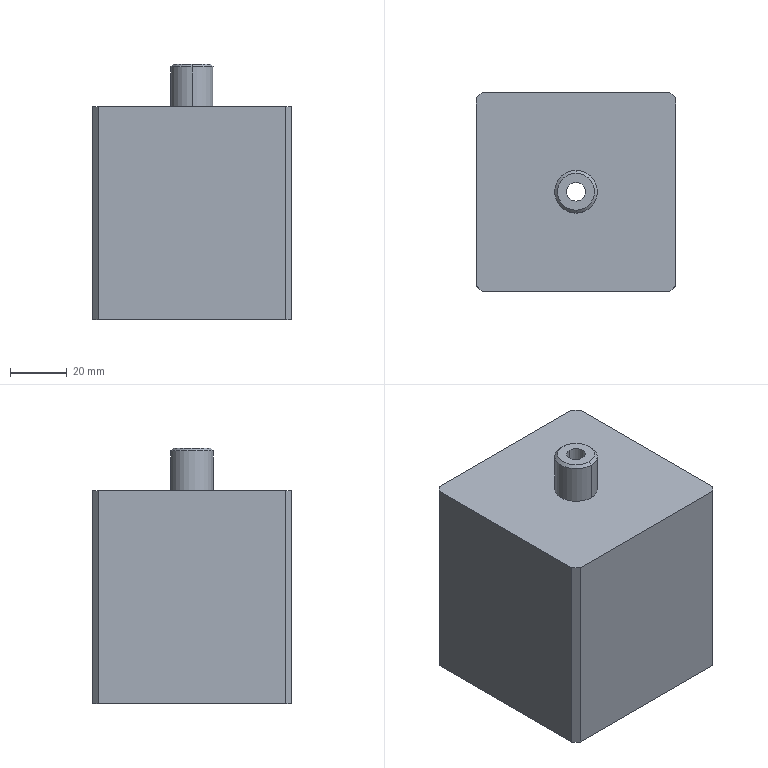NC program | NX | posted with a generic post | part box 70 x 70 x 90 mm
Lines 8020 to 8810 of 10206:
(ZLEVEL_PROFILE_COPY_1_COPY_COPY , TOOL : D6R3)
N16002 T23 M6
N16004 G54
N16006 G17 G0 G90 X-1.647 Y24.903 S7500 M3
N16008 G43 Z30. H23
N16010 Z1.4
N16012 G94 G1 X-3.316 Y24.789 Z1.312 F1000.
N16014 X-5.51 Y24.487 Z1.196
N16016 X-7.678 Y24.036 Z1.08
N16018 X-9.809 Y23.438 Z0.964
N16020 X-11.896 Y22.696 Z0.848
N16022 X-13.926 Y21.813 Z0.732
N16024 X-15.892 Y20.794 Z0.616
N16026 X-17.783 Y19.642 Z0.5
N16028 X-19.591 Y18.364 Z0.384
N16030 X-21.308 Y16.966 Z0.268
N16032 X-22.925 Y15.454 Z0.152
N16034 X-24.435 Y13.834 Z0.036
N16036 X-24.949 Y13.214 Z-0.006
N16038 Y-13.214 F2500.
N16040 G3 X24.949 Y-13.214 R32.389
N16042 G1 Y13.214
N16044 G3 X-24.949 Y13.214 R32.389
N16046 G1 X-24.914 Y13.108 Z-0.008
N16048 X-24.884 Y13.002 Z-0.01
N16050 X-24.856 Y12.896 Z-0.012
N16052 X-24.83 Y12.79 Z-0.014
N16054 Y-13.171
N16056 G3 X24.83 Y-13.171 R32.27
N16058 G1 Y13.171
N16060 G3 X-24.83 Y13.171 R32.27
N16062 G1 X-24.799 Y13.035 Z-0.016
N16064 X-24.77 Y12.898 Z-0.018
N16066 X-24.744 Y12.762 Z-0.021
N16068 X-24.718 Y12.625 Z-0.023
N16070 Y-13.131
N16072 G3 X24.718 Y-13.131 R32.159
N16074 G1 Y13.131
N16076 G3 X-24.718 Y13.131 R32.159
N16078 G1 X-24.689 Y12.965 Z-0.026
N16080 X-24.662 Y12.799 Z-0.029
N16082 X-24.636 Y12.634 Z-0.032
N16084 X-24.611 Y12.468 Z-0.035
N16086 Y-13.092
N16088 G3 X24.611 Y-13.092 R32.051
N16090 G1 Y13.092
N16092 G3 X-24.611 Y13.092 R32.051
N16094 G1 X-24.592 Y12.963 Z-0.037
N16096 X-24.574 Y12.835 Z-0.039
N16098 X-24.556 Y12.706 Z-0.042
N16100 X-24.539 Y12.577 Z-0.044
N16102 X-24.523 Y12.448 Z-0.046
N16104 X-24.506 Y12.319 Z-0.048
N16106 Y-13.054
N16108 G3 X24.506 Y-13.054 R31.947
N16110 G1 Y13.054
N16112 G3 X-24.506 Y13.054 R31.947
N16114 G1 X-24.488 Y12.906 Z-0.051
N16116 X-24.47 Y12.757 Z-0.054
N16118 X-24.453 Y12.608 Z-0.056
N16120 X-24.436 Y12.459 Z-0.059
N16122 X-24.419 Y12.311 Z-0.061
N16124 X-24.403 Y12.162 Z-0.064
N16126 Y-13.017
N16128 G3 X24.403 Y-13.017 R31.844
N16130 G1 Y13.017
N16132 G3 X-24.403 Y13.017 R31.844
N16134 G1 X-24.385 Y12.85 Z-0.067
N16136 X-24.368 Y12.683 Z-0.07
N16138 X-24.351 Y12.516 Z-0.073
N16140 X-24.334 Y12.349 Z-0.076
N16142 X-24.318 Y12.182 Z-0.078
N16144 X-24.302 Y12.015 Z-0.081
N16146 Y-12.98
N16148 G3 X24.302 Y-12.98 R31.742
N16150 G1 Y12.98
N16152 G3 X-24.302 Y12.98 R31.742
N16154 G1 X-24.288 Y12.84 Z-0.084
N16156 X-24.275 Y12.701 Z-0.086
N16158 X-24.262 Y12.561 Z-0.089
N16160 X-24.25 Y12.422 Z-0.091
N16162 X-24.237 Y12.282 Z-0.094
N16164 X-24.225 Y12.143 Z-0.096
N16166 X-24.213 Y12.003 Z-0.098
N16168 X-24.201 Y11.864 Z-0.101
N16170 Y-12.943
N16172 G3 X24.201 Y-12.943 R31.641
N16174 G1 Y12.943
N16176 G3 X-24.201 Y12.943 R31.641
N16178 G1 X-24.188 Y12.789 Z-0.104
N16180 X-24.175 Y12.636 Z-0.106
N16182 X-24.162 Y12.482 Z-0.109
N16184 X-24.15 Y12.328 Z-0.112
N16186 X-24.137 Y12.175 Z-0.114
N16188 X-24.125 Y12.021 Z-0.117
N16190 X-24.113 Y11.867 Z-0.12
N16192 X-24.101 Y11.713 Z-0.122
N16194 Y-12.907
N16196 G3 X24.101 Y-12.907 R31.541
N16198 G1 Y12.907
N16200 G3 X-24.101 Y12.907 R31.541
N16202 G1 X-24.088 Y12.739 Z-0.125
N16204 X-24.075 Y12.571 Z-0.128
N16206 X-24.063 Y12.404 Z-0.131
N16208 X-24.05 Y12.236 Z-0.134
N16210 X-24.038 Y12.069 Z-0.137
N16212 X-24.026 Y11.901 Z-0.14
N16214 X-24.014 Y11.734 Z-0.143
N16216 X-24.002 Y11.566 Z-0.146
N16218 Y-12.87
N16220 G3 X24.002 Y-12.87 R31.442
N16222 G1 Y12.87
N16224 G3 X-24.002 Y12.87 R31.442
N16226 G1 X-23.991 Y12.725 Z-0.148
N16228 X-23.981 Y12.58 Z-0.151
N16230 X-23.971 Y12.435 Z-0.153
N16232 X-23.961 Y12.29 Z-0.156
N16234 X-23.951 Y12.145 Z-0.158
N16236 X-23.942 Y12. Z-0.161
N16238 X-23.932 Y11.855 Z-0.163
N16240 X-23.922 Y11.71 Z-0.166
N16242 X-23.913 Y11.565 Z-0.169
N16244 X-23.903 Y11.42 Z-0.171
N16246 Y-12.834
N16248 G3 X23.903 Y-12.834 R31.344
N16250 G1 Y12.834
N16252 G3 X-23.903 Y12.834 R31.344
N16254 G1 X-23.893 Y12.678 Z-0.174
N16256 X-23.883 Y12.522 Z-0.176
N16258 X-23.873 Y12.366 Z-0.179
N16260 X-23.863 Y12.21 Z-0.182
N16262 X-23.854 Y12.053 Z-0.185
N16264 X-23.844 Y11.897 Z-0.187
N16266 X-23.834 Y11.741 Z-0.19
N16268 X-23.825 Y11.585 Z-0.193
N16270 X-23.815 Y11.429 Z-0.196
N16272 X-23.806 Y11.272 Z-0.198
N16274 Y-12.798
N16276 G3 X23.806 Y-12.798 R31.246
N16278 G1 Y12.798
N16280 G3 X-23.806 Y12.798 R31.246
N16282 G1 X-23.796 Y12.631 Z-0.201
N16284 X-23.786 Y12.464 Z-0.204
N16286 X-23.776 Y12.297 Z-0.207
N16288 X-23.766 Y12.13 Z-0.21
N16290 X-23.757 Y11.962 Z-0.213
N16292 X-23.747 Y11.795 Z-0.216
N16294 X-23.737 Y11.628 Z-0.219
N16296 X-23.728 Y11.461 Z-0.222
N16298 X-23.718 Y11.294 Z-0.225
N16300 X-23.709 Y11.126 Z-0.227
N16302 Y-12.763
N16304 G3 X23.709 Y-12.763 R31.149
N16306 G1 Y12.763
N16308 G3 X-23.709 Y12.763 R31.149
N16310 G1 X-23.701 Y12.614 Z-0.23
N16312 X-23.692 Y12.466 Z-0.233
N16314 X-23.684 Y12.318 Z-0.235
N16316 X-23.676 Y12.169 Z-0.238
N16318 X-23.668 Y12.021 Z-0.24
N16320 X-23.66 Y11.873 Z-0.243
N16322 X-23.652 Y11.724 Z-0.246
N16324 X-23.644 Y11.576 Z-0.248
N16326 X-23.636 Y11.427 Z-0.251
N16328 X-23.628 Y11.279 Z-0.253
N16330 X-23.621 Y11.131 Z-0.256
N16332 X-23.613 Y10.982 Z-0.259
N16334 Y-12.727
N16336 G3 X23.613 Y-12.727 R31.053
N16338 G1 Y12.727
N16340 G3 X-23.613 Y12.727 R31.053
N16342 G1 X-23.605 Y12.57 Z-0.261
N16344 X-23.597 Y12.412 Z-0.264
N16346 X-23.588 Y12.255 Z-0.267
N16348 X-23.58 Y12.097 Z-0.27
N16350 X-23.572 Y11.94 Z-0.272
N16352 X-23.564 Y11.782 Z-0.275
N16354 X-23.557 Y11.625 Z-0.278
N16356 X-23.549 Y11.467 Z-0.281
N16358 X-23.541 Y11.31 Z-0.283
N16360 X-23.533 Y11.152 Z-0.286
N16362 X-23.525 Y10.995 Z-0.289
N16364 X-23.518 Y10.837 Z-0.292
N16366 Y-12.692
N16368 G3 X23.518 Y-12.692 R30.958
N16370 G1 Y12.692
N16372 G3 X-23.518 Y12.692 R30.958
N16374 G1 X-23.509 Y12.526 Z-0.294
N16376 X-23.501 Y12.359 Z-0.297
N16378 X-23.493 Y12.193 Z-0.3
N16380 X-23.485 Y12.026 Z-0.303
N16382 X-23.477 Y11.86 Z-0.306
N16384 X-23.47 Y11.693 Z-0.309
N16386 X-23.462 Y11.527 Z-0.312
N16388 X-23.454 Y11.36 Z-0.315
N16390 X-23.446 Y11.194 Z-0.318
N16392 X-23.438 Y11.028 Z-0.321
N16394 X-23.431 Y10.861 Z-0.324
N16396 X-23.423 Y10.695 Z-0.326
N16398 Y-12.657
N16400 G3 X23.423 Y-12.657 R30.863
N16402 G1 Y12.657
N16404 G3 X-23.423 Y12.657 R30.863
N16406 G1 X-23.416 Y12.507 Z-0.329
N16408 X-23.409 Y12.357 Z-0.332
N16410 X-23.402 Y12.206 Z-0.334
N16412 X-23.396 Y12.056 Z-0.337
N16414 X-23.389 Y11.906 Z-0.34
N16416 X-23.382 Y11.755 Z-0.342
N16418 X-23.375 Y11.605 Z-0.345
N16420 X-23.369 Y11.455 Z-0.347
N16422 X-23.362 Y11.304 Z-0.35
N16424 X-23.355 Y11.154 Z-0.353
N16426 X-23.349 Y11.004 Z-0.355
N16428 X-23.342 Y10.853 Z-0.358
N16430 X-23.336 Y10.703 Z-0.361
N16432 X-23.329 Y10.553 Z-0.363
N16434 Y-12.622
N16436 G3 X23.329 Y-12.622 R30.77
N16438 G1 Y12.622
N16440 G3 X-23.329 Y12.622 R30.77
N16442 G1 X-23.322 Y12.465 Z-0.366
N16444 X-23.316 Y12.307 Z-0.369
N16446 X-23.309 Y12.149 Z-0.371
N16448 X-23.302 Y11.991 Z-0.374
N16450 X-23.295 Y11.833 Z-0.377
N16452 X-23.289 Y11.675 Z-0.38
N16454 X-23.282 Y11.517 Z-0.382
N16456 X-23.275 Y11.359 Z-0.385
N16458 X-23.269 Y11.202 Z-0.388
N16460 X-23.262 Y11.044 Z-0.391
N16462 X-23.256 Y10.886 Z-0.393
N16464 X-23.249 Y10.728 Z-0.396
N16466 X-23.243 Y10.57 Z-0.399
N16468 X-23.236 Y10.412 Z-0.402
N16470 Y-12.588
N16472 G3 X23.236 Y-12.588 R30.677
N16474 G1 Y12.588
N16476 G3 X-23.236 Y12.588 R30.677
N16478 G1 X-23.23 Y12.423 Z-0.405
N16480 X-23.223 Y12.257 Z-0.408
N16482 X-23.216 Y12.092 Z-0.41
N16484 X-23.209 Y11.926 Z-0.413
N16486 X-23.203 Y11.761 Z-0.416
N16488 X-23.196 Y11.595 Z-0.419
N16490 X-23.19 Y11.43 Z-0.422
N16492 X-23.183 Y11.265 Z-0.425
N16494 X-23.177 Y11.099 Z-0.428
N16496 X-23.17 Y10.934 Z-0.431
N16498 X-23.164 Y10.768 Z-0.434
N16500 X-23.157 Y10.603 Z-0.436
N16502 X-23.151 Y10.438 Z-0.439
N16504 X-23.144 Y10.272 Z-0.442
N16506 Y-12.554
N16508 G3 X23.144 Y-12.554 R30.585
N16510 G1 Y12.554
N16512 G3 X-23.144 Y12.554 R30.585
N16514 G1 X-23.138 Y12.381 Z-0.445
N16516 X-23.131 Y12.208 Z-0.448
N16518 X-23.124 Y12.035 Z-0.451
N16520 X-23.118 Y11.862 Z-0.454
N16522 X-23.111 Y11.689 Z-0.457
N16524 X-23.105 Y11.517 Z-0.46
N16526 X-23.098 Y11.344 Z-0.463
N16528 X-23.092 Y11.171 Z-0.466
N16530 X-23.085 Y10.998 Z-0.469
N16532 X-23.079 Y10.825 Z-0.472
N16534 X-23.072 Y10.652 Z-0.475
N16536 X-23.066 Y10.479 Z-0.478
N16538 X-23.059 Y10.306 Z-0.481
N16540 X-23.053 Y10.134 Z-0.484
N16542 Y-12.52
N16544 G3 X23.053 Y-12.52 R30.494
N16546 G1 Y12.52
N16548 G3 X-23.053 Y12.52 R30.494
N16550 G1 X-23.047 Y12.362 Z-0.487
N16552 X-23.041 Y12.204 Z-0.49
N16554 X-23.036 Y12.047 Z-0.493
N16556 X-23.03 Y11.889 Z-0.495
N16558 X-23.024 Y11.731 Z-0.498
N16560 X-23.019 Y11.574 Z-0.501
N16562 X-23.013 Y11.416 Z-0.504
N16564 X-23.007 Y11.258 Z-0.506
N16566 X-23.002 Y11.101 Z-0.509
N16568 X-22.996 Y10.943 Z-0.512
N16570 X-22.99 Y10.785 Z-0.515
N16572 X-22.985 Y10.628 Z-0.517
N16574 X-22.979 Y10.47 Z-0.52
N16576 X-22.974 Y10.312 Z-0.523
N16578 X-22.968 Y10.155 Z-0.526
N16580 X-22.963 Y9.997 Z-0.528
N16582 Y-12.486
N16584 G3 X22.963 Y-12.486 R30.403
N16586 G1 Y12.486
N16588 G3 X-22.963 Y12.486 R30.403
N16590 G1 X-22.957 Y12.322 Z-0.531
N16592 X-22.951 Y12.158 Z-0.534
N16594 X-22.946 Y11.994 Z-0.537
N16596 X-22.94 Y11.83 Z-0.54
N16598 X-22.934 Y11.665 Z-0.543
N16600 X-22.929 Y11.501 Z-0.546
N16602 X-22.923 Y11.337 Z-0.549
N16604 X-22.918 Y11.173 Z-0.551
N16606 X-22.912 Y11.009 Z-0.554
N16608 X-22.906 Y10.845 Z-0.557
N16610 X-22.901 Y10.681 Z-0.56
N16612 X-22.895 Y10.516 Z-0.563
N16614 X-22.89 Y10.352 Z-0.566
N16616 X-22.884 Y10.188 Z-0.569
N16618 X-22.879 Y10.024 Z-0.571
N16620 X-22.873 Y9.86 Z-0.574
N16622 Y-12.453
N16624 G3 X22.873 Y-12.453 R30.314
N16626 G1 Y12.453
N16628 G3 X-22.873 Y12.453 R30.314
N16630 G1 X-22.868 Y12.282 Z-0.577
N16632 X-22.862 Y12.112 Z-0.58
N16634 X-22.856 Y11.941 Z-0.583
N16636 X-22.851 Y11.771 Z-0.586
N16638 X-22.845 Y11.601 Z-0.589
N16640 X-22.84 Y11.43 Z-0.592
N16642 X-22.834 Y11.26 Z-0.595
N16644 X-22.829 Y11.089 Z-0.598
N16646 X-22.823 Y10.919 Z-0.601
N16648 X-22.818 Y10.748 Z-0.604
N16650 X-22.812 Y10.578 Z-0.607
N16652 X-22.807 Y10.407 Z-0.61
N16654 X-22.801 Y10.237 Z-0.613
N16656 X-22.796 Y10.067 Z-0.616
N16658 X-22.79 Y9.896 Z-0.619
N16660 X-22.785 Y9.726 Z-0.622
N16662 Y-12.42
N16664 G3 X22.785 Y-12.42 R30.225
N16666 G1 Y12.42
N16668 G3 X-22.785 Y12.42 R30.225
N16670 G1 X-22.78 Y12.263 Z-0.625
N16672 X-22.775 Y12.105 Z-0.627
N16674 X-22.77 Y11.948 Z-0.63
N16676 X-22.765 Y11.791 Z-0.633
N16678 X-22.76 Y11.634 Z-0.636
N16680 X-22.755 Y11.477 Z-0.638
N16682 X-22.751 Y11.32 Z-0.641
N16684 X-22.746 Y11.163 Z-0.644
N16686 X-22.741 Y11.006 Z-0.647
N16688 X-22.736 Y10.849 Z-0.649
N16690 X-22.731 Y10.692 Z-0.652
N16692 X-22.726 Y10.535 Z-0.655
N16694 X-22.721 Y10.378 Z-0.658
N16696 X-22.717 Y10.221 Z-0.66
N16698 X-22.712 Y10.064 Z-0.663
N16700 X-22.707 Y9.906 Z-0.666
N16702 X-22.702 Y9.749 Z-0.669
N16704 X-22.698 Y9.592 Z-0.671
N16706 Y-12.387
N16708 G3 X22.698 Y-12.387 R30.138
N16710 G1 Y12.387
N16712 G3 X-22.698 Y12.387 R30.138
N16714 G1 X-22.693 Y12.224 Z-0.674
N16716 X-22.688 Y12.062 Z-0.677
N16718 X-22.683 Y11.899 Z-0.68
N16720 X-22.678 Y11.737 Z-0.683
N16722 X-22.673 Y11.574 Z-0.685
N16724 X-22.668 Y11.411 Z-0.688
N16726 X-22.664 Y11.249 Z-0.691
N16728 X-22.659 Y11.086 Z-0.694
N16730 X-22.654 Y10.924 Z-0.697
N16732 X-22.649 Y10.761 Z-0.7
N16734 X-22.644 Y10.598 Z-0.702
N16736 X-22.64 Y10.436 Z-0.705
N16738 X-22.635 Y10.273 Z-0.708
N16740 X-22.63 Y10.111 Z-0.711
N16742 X-22.625 Y9.948 Z-0.714
N16744 X-22.621 Y9.786 Z-0.717
N16746 X-22.616 Y9.623 Z-0.719
N16748 X-22.611 Y9.46 Z-0.722
N16750 Y-12.354
N16752 G3 X22.611 Y-12.354 R30.052
N16754 G1 Y12.354
N16756 G3 X-22.611 Y12.354 R30.052
N16758 G1 X-22.606 Y12.186 Z-0.725
N16760 X-22.602 Y12.018 Z-0.728
N16762 X-22.597 Y11.85 Z-0.731
N16764 X-22.592 Y11.682 Z-0.734
N16766 X-22.587 Y11.514 Z-0.737
N16768 X-22.582 Y11.346 Z-0.74
N16770 X-22.578 Y11.178 Z-0.743
N16772 X-22.573 Y11.01 Z-0.746
N16774 X-22.568 Y10.842 Z-0.749
N16776 X-22.563 Y10.674 Z-0.752
N16778 X-22.559 Y10.506 Z-0.755
N16780 X-22.554 Y10.338 Z-0.758
N16782 X-22.549 Y10.17 Z-0.76
N16784 X-22.545 Y10.002 Z-0.763
N16786 X-22.54 Y9.834 Z-0.766
N16788 X-22.535 Y9.666 Z-0.769
N16790 X-22.531 Y9.498 Z-0.772
N16792 X-22.526 Y9.33 Z-0.775
N16794 Y-12.322
N16796 G3 X22.526 Y-12.322 R29.966
N16798 G1 Y12.322
N16800 G3 X-22.526 Y12.322 R29.966
N16802 G1 X-22.522 Y12.166 Z-0.778
N16804 X-22.517 Y12.01 Z-0.781
N16806 X-22.513 Y11.854 Z-0.783
N16808 X-22.509 Y11.698 Z-0.786
N16810 X-22.505 Y11.542 Z-0.789
N16812 X-22.5 Y11.386 Z-0.791
N16814 X-22.496 Y11.23 Z-0.794
N16816 X-22.492 Y11.074 Z-0.797
N16818 X-22.488 Y10.918 Z-0.8
N16820 X-22.483 Y10.762 Z-0.802
N16822 X-22.479 Y10.606 Z-0.805
N16824 X-22.475 Y10.45 Z-0.808
N16826 X-22.471 Y10.294 Z-0.811
N16828 X-22.467 Y10.138 Z-0.813
N16830 X-22.462 Y9.982 Z-0.816
N16832 X-22.458 Y9.826 Z-0.819
N16834 X-22.454 Y9.67 Z-0.821
N16836 X-22.45 Y9.514 Z-0.824
N16838 X-22.446 Y9.358 Z-0.827
N16840 X-22.442 Y9.201 Z-0.83
N16842 Y-12.291
N16844 G3 X22.442 Y-12.291 R29.882
N16846 G1 Y12.291
N16848 G3 X-22.442 Y12.291 R29.882
N16850 G1 X-22.438 Y12.13 Z-0.832
N16852 X-22.433 Y11.969 Z-0.835
N16854 X-22.429 Y11.808 Z-0.838
N16856 X-22.425 Y11.647 Z-0.841
N16858 X-22.421 Y11.486 Z-0.844
N16860 X-22.416 Y11.326 Z-0.846
N16862 X-22.412 Y11.165 Z-0.849
N16864 X-22.408 Y11.004 Z-0.852
N16866 X-22.404 Y10.843 Z-0.855
N16868 X-22.4 Y10.682 Z-0.858
N16870 X-22.396 Y10.521 Z-0.86
N16872 X-22.392 Y10.361 Z-0.863
N16874 X-22.387 Y10.2 Z-0.866
N16876 X-22.383 Y10.039 Z-0.869
N16878 X-22.379 Y9.878 Z-0.872
N16880 X-22.375 Y9.717 Z-0.875
N16882 X-22.371 Y9.557 Z-0.877
N16884 X-22.367 Y9.396 Z-0.88
N16886 X-22.363 Y9.235 Z-0.883
N16888 X-22.359 Y9.074 Z-0.886
N16890 Y-12.259
N16892 G3 X22.359 Y-12.259 R29.799
N16894 G1 Y12.259
N16896 G3 X-22.359 Y12.259 R29.799
N16898 G1 X-22.355 Y12.094 Z-0.889
N16900 X-22.35 Y11.928 Z-0.892
N16902 X-22.346 Y11.763 Z-0.894
N16904 X-22.342 Y11.597 Z-0.897
N16906 X-22.338 Y11.432 Z-0.9
N16908 X-22.334 Y11.266 Z-0.903
N16910 X-22.33 Y11.101 Z-0.906
N16912 X-22.326 Y10.935 Z-0.909
N16914 X-22.321 Y10.769 Z-0.912
N16916 X-22.317 Y10.604 Z-0.915
N16918 X-22.313 Y10.438 Z-0.918
N16920 X-22.309 Y10.273 Z-0.92
N16922 X-22.305 Y10.107 Z-0.923
N16924 X-22.301 Y9.942 Z-0.926
N16926 X-22.297 Y9.776 Z-0.929
N16928 X-22.293 Y9.611 Z-0.932
N16930 X-22.289 Y9.445 Z-0.935
N16932 X-22.285 Y9.28 Z-0.938
N16934 X-22.281 Y9.114 Z-0.941
N16936 X-22.277 Y8.949 Z-0.944
N16938 Y-12.228
N16940 G3 X22.277 Y-12.228 R29.717
N16942 G1 Y12.228
N16944 G3 X-22.277 Y12.228 R29.717
N16946 G1 X-22.273 Y12.058 Z-0.946
N16948 X-22.269 Y11.888 Z-0.949
N16950 X-22.264 Y11.718 Z-0.952
N16952 X-22.26 Y11.548 Z-0.955
N16954 X-22.256 Y11.377 Z-0.958
N16956 X-22.252 Y11.207 Z-0.961
N16958 X-22.248 Y11.037 Z-0.964
N16960 X-22.244 Y10.867 Z-0.967
N16962 X-22.24 Y10.697 Z-0.97
N16964 X-22.236 Y10.527 Z-0.973
N16966 X-22.232 Y10.356 Z-0.976
N16968 X-22.228 Y10.186 Z-0.979
N16970 X-22.224 Y10.016 Z-0.982
N16972 X-22.22 Y9.846 Z-0.985
N16974 X-22.216 Y9.676 Z-0.988
N16976 X-22.212 Y9.506 Z-0.991
N16978 X-22.208 Y9.335 Z-0.994
N16980 X-22.204 Y9.165 Z-0.997
N16982 X-22.2 Y8.995 Z-1.
N16984 X-22.196 Y8.825 Z-1.003
N16986 Y-12.198
N16988 G3 X22.196 Y-12.198 R29.637
N16990 G1 Y12.198
N16992 G3 X-22.196 Y12.198 R29.637
N16994 G1 X-22.192 Y12.039 Z-1.006
N16996 X-22.189 Y11.88 Z-1.008
N16998 X-22.185 Y11.721 Z-1.011
N17000 X-22.181 Y11.562 Z-1.014
N17002 X-22.178 Y11.403 Z-1.017
N17004 X-22.174 Y11.245 Z-1.02
N17006 X-22.17 Y11.086 Z-1.022
N17008 X-22.167 Y10.927 Z-1.025
N17010 X-22.163 Y10.768 Z-1.028
N17012 X-22.16 Y10.609 Z-1.031
N17014 X-22.156 Y10.45 Z-1.033
N17016 X-22.152 Y10.291 Z-1.036
N17018 X-22.149 Y10.133 Z-1.039
N17020 X-22.145 Y9.974 Z-1.042
N17022 X-22.142 Y9.815 Z-1.045
N17024 X-22.138 Y9.656 Z-1.047
N17026 X-22.134 Y9.497 Z-1.05
N17028 X-22.131 Y9.338 Z-1.053
N17030 X-22.127 Y9.179 Z-1.056
N17032 X-22.124 Y9.021 Z-1.058
N17034 X-22.12 Y8.862 Z-1.061
N17036 X-22.117 Y8.703 Z-1.064
N17038 Y-12.168
N17040 G3 X22.117 Y-12.168 R29.557
N17042 G1 Y12.168
N17044 G3 X-22.117 Y12.168 R29.557
N17046 G1 X-22.113 Y12.005 Z-1.067
N17048 X-22.109 Y11.842 Z-1.07
N17050 X-22.106 Y11.679 Z-1.072
N17052 X-22.102 Y11.516 Z-1.075
N17054 X-22.099 Y11.353 Z-1.078
N17056 X-22.095 Y11.19 Z-1.081
N17058 X-22.091 Y11.027 Z-1.084
N17060 X-22.088 Y10.864 Z-1.087
N17062 X-22.084 Y10.701 Z-1.09
N17064 X-22.081 Y10.538 Z-1.092
N17066 X-22.077 Y10.375 Z-1.095
N17068 X-22.074 Y10.212 Z-1.098
N17070 X-22.07 Y10.049 Z-1.101
N17072 X-22.066 Y9.886 Z-1.104
N17074 X-22.063 Y9.723 Z-1.107
N17076 X-22.059 Y9.56 Z-1.109
N17078 X-22.056 Y9.397 Z-1.112
N17080 X-22.052 Y9.234 Z-1.115
N17082 X-22.049 Y9.072 Z-1.118
N17084 X-22.045 Y8.909 Z-1.121
N17086 X-22.042 Y8.746 Z-1.124
N17088 X-22.038 Y8.583 Z-1.127
N17090 Y-12.138
N17092 G3 X22.038 Y-12.138 R29.479
N17094 G1 Y12.138
N17096 G3 X-22.038 Y12.138 R29.479
N17098 G1 X-22.035 Y11.971 Z-1.129
N17100 X-22.031 Y11.804 Z-1.132
N17102 X-22.028 Y11.637 Z-1.135
N17104 X-22.024 Y11.47 Z-1.138
N17106 X-22.021 Y11.303 Z-1.141
N17108 X-22.017 Y11.136 Z-1.144
N17110 X-22.014 Y10.969 Z-1.147
N17112 X-22.01 Y10.802 Z-1.15
N17114 X-22.006 Y10.635 Z-1.153
N17116 X-22.003 Y10.468 Z-1.156
N17118 X-21.999 Y10.301 Z-1.159
N17120 X-21.996 Y10.134 Z-1.161
N17122 X-21.992 Y9.967 Z-1.164
N17124 X-21.989 Y9.8 Z-1.167
N17126 X-21.986 Y9.633 Z-1.17
N17128 X-21.982 Y9.466 Z-1.173
N17130 X-21.979 Y9.299 Z-1.176
N17132 X-21.975 Y9.132 Z-1.179
N17134 X-21.972 Y8.965 Z-1.182
N17136 X-21.968 Y8.798 Z-1.185
N17138 X-21.965 Y8.631 Z-1.188
N17140 X-21.961 Y8.464 Z-1.191
N17142 Y-12.109
N17144 G3 X21.961 Y-12.109 R29.402
N17146 G1 Y12.109
N17148 G3 X-21.961 Y12.109 R29.402
N17150 G1 X-21.958 Y11.938 Z-1.194
N17152 X-21.954 Y11.767 Z-1.197
N17154 X-21.951 Y11.596 Z-1.2
N17156 X-21.947 Y11.425 Z-1.203
N17158 X-21.944 Y11.254 Z-1.206
N17160 X-21.94 Y11.083 Z-1.209
N17162 X-21.937 Y10.912 Z-1.212
N17164 X-21.933 Y10.741 Z-1.215
N17166 X-21.93 Y10.57 Z-1.217
N17168 X-21.927 Y10.399 Z-1.22
N17170 X-21.923 Y10.228 Z-1.223
N17172 X-21.92 Y10.057 Z-1.226
N17174 X-21.916 Y9.886 Z-1.229
N17176 X-21.913 Y9.715 Z-1.232
N17178 X-21.909 Y9.544 Z-1.235
N17180 X-21.906 Y9.373 Z-1.238
N17182 X-21.903 Y9.203 Z-1.241
N17184 X-21.899 Y9.032 Z-1.244
N17186 X-21.896 Y8.861 Z-1.247
N17188 X-21.892 Y8.69 Z-1.25
N17190 X-21.889 Y8.519 Z-1.253
N17192 X-21.886 Y8.348 Z-1.256
N17194 Y-12.08
N17196 G3 X21.886 Y-12.08 R29.326
N17198 G1 Y12.08
N17200 G3 X-21.886 Y12.08 R29.326
N17202 G1 X-21.883 Y11.92 Z-1.259
N17204 X-21.879 Y11.759 Z-1.262
N17206 X-21.876 Y11.599 Z-1.265
N17208 X-21.873 Y11.439 Z-1.267
N17210 X-21.87 Y11.278 Z-1.27
N17212 X-21.867 Y11.118 Z-1.273
N17214 X-21.864 Y10.958 Z-1.276
N17216 X-21.861 Y10.798 Z-1.279
N17218 X-21.857 Y10.637 Z-1.281
N17220 X-21.854 Y10.477 Z-1.284
N17222 X-21.851 Y10.317 Z-1.287
N17224 X-21.848 Y10.156 Z-1.29
N17226 X-21.845 Y9.996 Z-1.293
N17228 X-21.842 Y9.836 Z-1.295
N17230 X-21.839 Y9.676 Z-1.298
N17232 X-21.836 Y9.515 Z-1.301
N17234 X-21.833 Y9.355 Z-1.304
N17236 X-21.83 Y9.195 Z-1.307
N17238 X-21.827 Y9.035 Z-1.309
N17240 X-21.824 Y8.874 Z-1.312
N17242 X-21.82 Y8.714 Z-1.315
N17244 X-21.817 Y8.554 Z-1.318
N17246 X-21.814 Y8.393 Z-1.321
N17248 X-21.811 Y8.233 Z-1.323
N17250 Y-12.051
N17252 G3 X21.811 Y-12.051 R29.252
N17254 G1 Y12.051
N17256 G3 X-21.811 Y12.051 R29.252
N17258 G1 X-21.808 Y11.888 Z-1.326
N17260 X-21.805 Y11.724 Z-1.329
N17262 X-21.802 Y11.56 Z-1.332
N17264 X-21.799 Y11.396 Z-1.335
N17266 X-21.796 Y11.233 Z-1.338
N17268 X-21.793 Y11.069 Z-1.341
N17270 X-21.79 Y10.905 Z-1.343
N17272 X-21.787 Y10.741 Z-1.346
N17274 X-21.784 Y10.577 Z-1.349
N17276 X-21.781 Y10.414 Z-1.352
N17278 X-21.778 Y10.25 Z-1.355
N17280 X-21.775 Y10.086 Z-1.358
N17282 X-21.771 Y9.922 Z-1.361
N17284 X-21.768 Y9.759 Z-1.363
N17286 X-21.765 Y9.595 Z-1.366
N17288 X-21.762 Y9.431 Z-1.369
N17290 X-21.759 Y9.267 Z-1.372
N17292 X-21.756 Y9.103 Z-1.375
N17294 X-21.753 Y8.94 Z-1.378
N17296 X-21.75 Y8.776 Z-1.381
N17298 X-21.747 Y8.612 Z-1.383
N17300 X-21.744 Y8.448 Z-1.386
N17302 X-21.741 Y8.285 Z-1.389
N17304 X-21.738 Y8.121 Z-1.392
N17306 Y-12.024
N17308 G3 X21.738 Y-12.024 R29.179
N17310 G1 Y12.024
N17312 G3 X-21.738 Y12.024 R29.179
N17314 G1 X-21.735 Y11.856 Z-1.395
N17316 X-21.732 Y11.689 Z-1.398
N17318 X-21.729 Y11.522 Z-1.401
N17320 X-21.726 Y11.355 Z-1.404
N17322 X-21.723 Y11.187 Z-1.407
N17324 X-21.72 Y11.02 Z-1.41
N17326 X-21.717 Y10.853 Z-1.412
N17328 X-21.714 Y10.686 Z-1.415
N17330 X-21.711 Y10.519 Z-1.418
N17332 X-21.708 Y10.351 Z-1.421
N17334 X-21.705 Y10.184 Z-1.424
N17336 X-21.702 Y10.017 Z-1.427
N17338 X-21.699 Y9.85 Z-1.43
N17340 X-21.696 Y9.683 Z-1.433
N17342 X-21.693 Y9.515 Z-1.436
N17344 X-21.69 Y9.348 Z-1.439
N17346 X-21.687 Y9.181 Z-1.442
N17348 X-21.684 Y9.014 Z-1.445
N17350 X-21.682 Y8.846 Z-1.447
N17352 X-21.679 Y8.679 Z-1.45
N17354 X-21.676 Y8.512 Z-1.453
N17356 X-21.673 Y8.345 Z-1.456
N17358 X-21.67 Y8.178 Z-1.459
N17360 X-21.667 Y8.01 Z-1.462
N17362 Y-11.996
N17364 G3 X21.667 Y-11.996 R29.107
N17366 G1 Y11.996
N17368 G3 X-21.667 Y11.996 R29.107
N17370 G1 X-21.664 Y11.826 Z-1.465
N17372 X-21.661 Y11.655 Z-1.468
N17374 X-21.658 Y11.484 Z-1.471
N17376 X-21.655 Y11.314 Z-1.474
N17378 X-21.652 Y11.143 Z-1.477
N17380 X-21.649 Y10.973 Z-1.48
N17382 X-21.646 Y10.802 Z-1.483
N17384 X-21.643 Y10.631 Z-1.486
N17386 X-21.64 Y10.461 Z-1.489
N17388 X-21.637 Y10.29 Z-1.492
N17390 X-21.634 Y10.12 Z-1.495
N17392 X-21.631 Y9.949 Z-1.498
N17394 X-21.629 Y9.779 Z-1.501
N17396 X-21.626 Y9.608 Z-1.504
N17398 X-21.623 Y9.437 Z-1.507
N17400 X-21.62 Y9.267 Z-1.51
N17402 X-21.617 Y9.096 Z-1.513
N17404 X-21.614 Y8.926 Z-1.516
N17406 X-21.611 Y8.755 Z-1.519
N17408 X-21.608 Y8.584 Z-1.522
N17410 X-21.605 Y8.414 Z-1.525
N17412 X-21.602 Y8.243 Z-1.528
N17414 X-21.6 Y8.073 Z-1.531
N17416 X-21.597 Y7.902 Z-1.534
N17418 Y-11.969
N17420 G3 X21.597 Y-11.969 R29.037
N17422 G1 Y11.969
N17424 G3 X-21.597 Y11.969 R29.037
N17426 G1 X-21.594 Y11.809 Z-1.536
N17428 X-21.591 Y11.648 Z-1.539
N17430 X-21.589 Y11.488 Z-1.542
N17432 X-21.586 Y11.327 Z-1.545
N17434 X-21.583 Y11.167 Z-1.548
N17436 X-21.581 Y11.006 Z-1.55
N17438 X-21.578 Y10.846 Z-1.553
N17440 X-21.575 Y10.685 Z-1.556
N17442 X-21.573 Y10.525 Z-1.559
N17444 X-21.57 Y10.364 Z-1.562
N17446 X-21.567 Y10.204 Z-1.564
N17448 X-21.565 Y10.043 Z-1.567
N17450 X-21.562 Y9.883 Z-1.57
N17452 X-21.559 Y9.722 Z-1.573
N17454 X-21.557 Y9.562 Z-1.576
N17456 X-21.554 Y9.401 Z-1.578
N17458 X-21.551 Y9.241 Z-1.581
N17460 X-21.549 Y9.08 Z-1.584
N17462 X-21.546 Y8.92 Z-1.587
N17464 X-21.544 Y8.759 Z-1.59
N17466 X-21.541 Y8.599 Z-1.592
N17468 X-21.538 Y8.438 Z-1.595
N17470 X-21.536 Y8.277 Z-1.598
N17472 X-21.533 Y8.117 Z-1.601
N17474 X-21.531 Y7.956 Z-1.604
N17476 X-21.528 Y7.796 Z-1.606
N17478 Y-11.943
N17480 G3 X21.528 Y-11.943 R28.968
N17482 G1 Y11.943
N17484 G3 X-21.528 Y11.943 R28.968
N17486 G1 X-21.525 Y11.779 Z-1.609
N17488 X-21.523 Y11.616 Z-1.612
N17490 X-21.52 Y11.452 Z-1.615
N17492 X-21.517 Y11.289 Z-1.618
N17494 X-21.515 Y11.125 Z-1.621
N17496 X-21.512 Y10.962 Z-1.624
N17498 X-21.51 Y10.798 Z-1.626
N17500 X-21.507 Y10.635 Z-1.629
N17502 X-21.504 Y10.471 Z-1.632
N17504 X-21.502 Y10.308 Z-1.635
N17506 X-21.499 Y10.144 Z-1.638
N17508 X-21.497 Y9.981 Z-1.641
N17510 X-21.494 Y9.817 Z-1.644
N17512 X-21.491 Y9.654 Z-1.646
N17514 X-21.489 Y9.49 Z-1.649
N17516 X-21.486 Y9.327 Z-1.652
N17518 X-21.484 Y9.163 Z-1.655
N17520 X-21.481 Y9. Z-1.658
N17522 X-21.479 Y8.836 Z-1.661
N17524 X-21.476 Y8.673 Z-1.663
N17526 X-21.474 Y8.509 Z-1.666
N17528 X-21.471 Y8.346 Z-1.669
N17530 X-21.468 Y8.182 Z-1.672
N17532 X-21.466 Y8.019 Z-1.675
N17534 X-21.463 Y7.855 Z-1.678
N17536 X-21.461 Y7.692 Z-1.681
N17538 Y-11.917
N17540 G3 X21.461 Y-11.917 R28.901
N17542 G1 Y11.917
N17544 G3 X-21.461 Y11.917 R28.901
N17546 G1 X-21.458 Y11.751 Z-1.684
N17548 X-21.456 Y11.584 Z-1.686
N17550 X-21.453 Y11.418 Z-1.689
N17552 X-21.451 Y11.251 Z-1.692
N17554 X-21.448 Y11.085 Z-1.695
N17556 X-21.445 Y10.919 Z-1.698
N17558 X-21.443 Y10.752 Z-1.701
N17560 X-21.44 Y10.586 Z-1.704
N17562 X-21.438 Y10.419 Z-1.707
N17564 X-21.435 Y10.253 Z-1.71
N17566 X-21.433 Y10.087 Z-1.713
N17568 X-21.43 Y9.92 Z-1.715
N17570 X-21.428 Y9.754 Z-1.718
N17572 X-21.425 Y9.587 Z-1.721
N17574 X-21.423 Y9.421 Z-1.724
N17576 X-21.42 Y9.254 Z-1.727